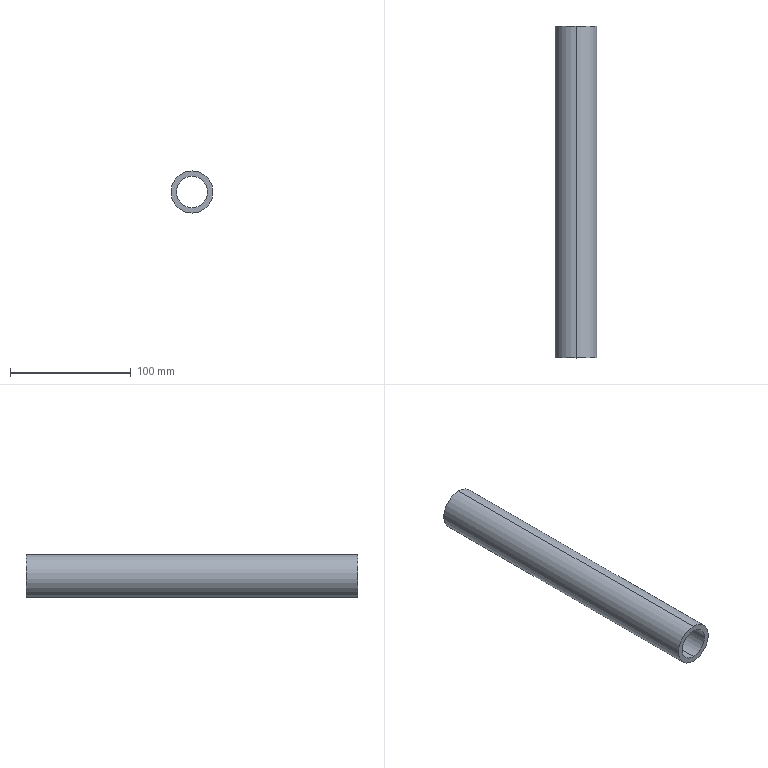Part | SolidWorks | features Extrusion 1, Shell 1 | 1 solid | 6 faces | box 35 x 275 x 35 mm | volume 118575 mm3 | cylinder 4 | plane 2 | commonest cylinder face diameters 26 x2 35 x2
STEP:
#1=CARTESIAN_POINT('',(0.,275.,-13.));
#2=VERTEX_POINT('',#1);
#3=CARTESIAN_POINT('',(0.,275.,13.));
#4=VERTEX_POINT('',#3);
#5=CARTESIAN_POINT('',(0.,275.,0.));
#6=DIRECTION('',(0.,1.,0.));
#7=DIRECTION('',(0.,0.,1.));
#8=AXIS2_PLACEMENT_3D('',#5,#6,#7);
#9=CIRCLE('',#8,13.);
#10=EDGE_CURVE('',#2,#4,#9,.T.);
#11=ORIENTED_EDGE('',*,*,#10,.T.);
#12=CARTESIAN_POINT('',(0.,0.,13.));
#13=VERTEX_POINT('',#12);
#14=CARTESIAN_POINT('',(0.,275.,13.));
#15=DIRECTION('',(0.,-1.,0.));
#16=VECTOR('',#15,1000.);
#17=LINE('',#14,#16);
#18=EDGE_CURVE('',#4,#13,#17,.T.);
#19=ORIENTED_EDGE('',*,*,#18,.T.);
#20=CARTESIAN_POINT('',(0.,0.,-13.));
#21=VERTEX_POINT('',#20);
#22=CARTESIAN_POINT('',(0.,0.,0.));
#23=DIRECTION('',(0.,1.,0.));
#24=DIRECTION('',(0.,0.,1.));
#25=AXIS2_PLACEMENT_3D('',#22,#23,#24);
#26=CIRCLE('',#25,13.);
#27=EDGE_CURVE('',#21,#13,#26,.T.);
#28=ORIENTED_EDGE('',*,*,#27,.F.);
#29=CARTESIAN_POINT('',(0.,275.,-13.));
#30=DIRECTION('',(0.,-1.,0.));
#31=VECTOR('',#30,1000.);
#32=LINE('',#29,#31);
#33=EDGE_CURVE('',#2,#21,#32,.T.);
#34=ORIENTED_EDGE('',*,*,#33,.F.);
#35=EDGE_LOOP('',(#11,#19,#28,#34));
#36=FACE_OUTER_BOUND('',#35,.T.);
#37=CARTESIAN_POINT('',(0.,275.,0.));
#38=DIRECTION('',(0.,-1.,0.));
#39=DIRECTION('',(0.,0.,-1.));
#40=AXIS2_PLACEMENT_3D('',#37,#38,#39);
#41=CYLINDRICAL_SURFACE('',#40,13.);
#42=ADVANCED_FACE('',(#36),#41,.F.);
#43=CARTESIAN_POINT('',(0.,275.,17.5));
#44=VERTEX_POINT('',#43);
#45=CARTESIAN_POINT('',(0.,275.,-17.5));
#46=VERTEX_POINT('',#45);
#47=CARTESIAN_POINT('',(0.,275.,0.));
#48=DIRECTION('',(0.,1.,0.));
#49=DIRECTION('',(0.,0.,1.));
#50=AXIS2_PLACEMENT_3D('',#47,#48,#49);
#51=CIRCLE('',#50,17.5);
#52=EDGE_CURVE('',#44,#46,#51,.T.);
#53=ORIENTED_EDGE('',*,*,#52,.F.);
#54=CARTESIAN_POINT('',(0.,0.,17.5));
#55=VERTEX_POINT('',#54);
#56=CARTESIAN_POINT('',(0.,275.,17.5));
#57=DIRECTION('',(0.,-1.,0.));
#58=VECTOR('',#57,1000.);
#59=LINE('',#56,#58);
#60=EDGE_CURVE('',#44,#55,#59,.T.);
#61=ORIENTED_EDGE('',*,*,#60,.T.);
#62=CARTESIAN_POINT('',(0.,0.,-17.5));
#63=VERTEX_POINT('',#62);
#64=CARTESIAN_POINT('',(0.,0.,0.));
#65=DIRECTION('',(0.,1.,0.));
#66=DIRECTION('',(0.,0.,1.));
#67=AXIS2_PLACEMENT_3D('',#64,#65,#66);
#68=CIRCLE('',#67,17.5);
#69=EDGE_CURVE('',#55,#63,#68,.T.);
#70=ORIENTED_EDGE('',*,*,#69,.T.);
#71=CARTESIAN_POINT('',(0.,275.,-17.5));
#72=DIRECTION('',(0.,-1.,0.));
#73=VECTOR('',#72,1000.);
#74=LINE('',#71,#73);
#75=EDGE_CURVE('',#46,#63,#74,.T.);
#76=ORIENTED_EDGE('',*,*,#75,.F.);
#77=EDGE_LOOP('',(#53,#61,#70,#76));
#78=FACE_OUTER_BOUND('',#77,.T.);
#79=CARTESIAN_POINT('',(0.,275.,0.));
#80=DIRECTION('',(0.,-1.,0.));
#81=DIRECTION('',(0.,0.,-1.));
#82=AXIS2_PLACEMENT_3D('',#79,#80,#81);
#83=CYLINDRICAL_SURFACE('',#82,17.5);
#84=ADVANCED_FACE('',(#78),#83,.T.);
#85=ORIENTED_EDGE('',*,*,#60,.F.);
#86=CARTESIAN_POINT('',(0.,275.,0.));
#87=DIRECTION('',(0.,1.,0.));
#88=DIRECTION('',(0.,0.,1.));
#89=AXIS2_PLACEMENT_3D('',#86,#87,#88);
#90=CIRCLE('',#89,17.5);
#91=EDGE_CURVE('',#46,#44,#90,.T.);
#92=ORIENTED_EDGE('',*,*,#91,.F.);
#93=ORIENTED_EDGE('',*,*,#75,.T.);
#94=CARTESIAN_POINT('',(0.,0.,0.));
#95=DIRECTION('',(0.,1.,0.));
#96=DIRECTION('',(0.,0.,1.));
#97=AXIS2_PLACEMENT_3D('',#94,#95,#96);
#98=CIRCLE('',#97,17.5);
#99=EDGE_CURVE('',#63,#55,#98,.T.);
#100=ORIENTED_EDGE('',*,*,#99,.T.);
#101=EDGE_LOOP('',(#85,#92,#93,#100));
#102=FACE_OUTER_BOUND('',#101,.T.);
#103=CARTESIAN_POINT('',(0.,275.,0.));
#104=DIRECTION('',(0.,-1.,0.));
#105=DIRECTION('',(0.,0.,-1.));
#106=AXIS2_PLACEMENT_3D('',#103,#104,#105);
#107=CYLINDRICAL_SURFACE('',#106,17.5);
#108=ADVANCED_FACE('',(#102),#107,.T.);
#109=ORIENTED_EDGE('',*,*,#10,.F.);
#110=CARTESIAN_POINT('',(0.,275.,0.));
#111=DIRECTION('',(0.,1.,0.));
#112=DIRECTION('',(0.,0.,1.));
#113=AXIS2_PLACEMENT_3D('',#110,#111,#112);
#114=CIRCLE('',#113,13.);
#115=EDGE_CURVE('',#4,#2,#114,.T.);
#116=ORIENTED_EDGE('',*,*,#115,.F.);
#117=EDGE_LOOP('',(#109,#116));
#118=FACE_BOUND('',#117,.T.);
#119=ORIENTED_EDGE('',*,*,#91,.T.);
#120=ORIENTED_EDGE('',*,*,#52,.T.);
#121=EDGE_LOOP('',(#119,#120));
#122=FACE_OUTER_BOUND('',#121,.T.);
#123=CARTESIAN_POINT('',(0.,275.,0.));
#124=DIRECTION('',(0.,1.,0.));
#125=DIRECTION('',(0.,0.,1.));
#126=AXIS2_PLACEMENT_3D('',#123,#124,#125);
#127=PLANE('',#126);
#128=ADVANCED_FACE('',(#118,#122),#127,.T.);
#129=ORIENTED_EDGE('',*,*,#27,.T.);
#130=CARTESIAN_POINT('',(0.,0.,0.));
#131=DIRECTION('',(0.,1.,0.));
#132=DIRECTION('',(0.,0.,1.));
#133=AXIS2_PLACEMENT_3D('',#130,#131,#132);
#134=CIRCLE('',#133,13.);
#135=EDGE_CURVE('',#13,#21,#134,.T.);
#136=ORIENTED_EDGE('',*,*,#135,.T.);
#137=EDGE_LOOP('',(#129,#136));
#138=FACE_BOUND('',#137,.T.);
#139=ORIENTED_EDGE('',*,*,#99,.F.);
#140=ORIENTED_EDGE('',*,*,#69,.F.);
#141=EDGE_LOOP('',(#139,#140));
#142=FACE_OUTER_BOUND('',#141,.T.);
#143=CARTESIAN_POINT('',(0.,0.,0.));
#144=DIRECTION('',(0.,1.,0.));
#145=DIRECTION('',(0.,0.,1.));
#146=AXIS2_PLACEMENT_3D('',#143,#144,#145);
#147=PLANE('',#146);
#148=ADVANCED_FACE('',(#138,#142),#147,.F.);
#149=ORIENTED_EDGE('',*,*,#18,.F.);
#150=ORIENTED_EDGE('',*,*,#115,.T.);
#151=ORIENTED_EDGE('',*,*,#33,.T.);
#152=ORIENTED_EDGE('',*,*,#135,.F.);
#153=EDGE_LOOP('',(#149,#150,#151,#152));
#154=FACE_OUTER_BOUND('',#153,.T.);
#155=CARTESIAN_POINT('',(0.,275.,0.));
#156=DIRECTION('',(0.,-1.,0.));
#157=DIRECTION('',(0.,0.,-1.));
#158=AXIS2_PLACEMENT_3D('',#155,#156,#157);
#159=CYLINDRICAL_SURFACE('',#158,13.);
#160=ADVANCED_FACE('',(#154),#159,.F.);
#161=CLOSED_SHELL('',(#42,#84,#108,#128,#148,#160));
#162=MANIFOLD_SOLID_BREP('',#161);
#163=CARTESIAN_POINT('',(0.,0.,0.));
#164=DIRECTION('',(0.,0.,1.));
#165=DIRECTION('',(1.,0.,0.));
#166=AXIS2_PLACEMENT_3D('',#163,#164,#165);
#167=(LENGTH_UNIT()NAMED_UNIT(*)SI_UNIT(.MILLI.,.METRE.));
#168=UNCERTAINTY_MEASURE_WITH_UNIT(LENGTH_MEASURE(0.00001),#167,'','');
#169=(NAMED_UNIT(*)PLANE_ANGLE_UNIT()SI_UNIT($,.RADIAN.));
#170=(NAMED_UNIT(*)SI_UNIT($,.STERADIAN.)SOLID_ANGLE_UNIT());
#171=(GEOMETRIC_REPRESENTATION_CONTEXT(3)GLOBAL_UNCERTAINTY_ASSIGNED_CONTEXT((#168))GLOBAL_UNIT_ASSIGNED_CONTEXT((#167,#169,#170))REPRESENTATION_CONTEXT('',''));
#172=ADVANCED_BREP_SHAPE_REPRESENTATION('',(#162,#166),#171);